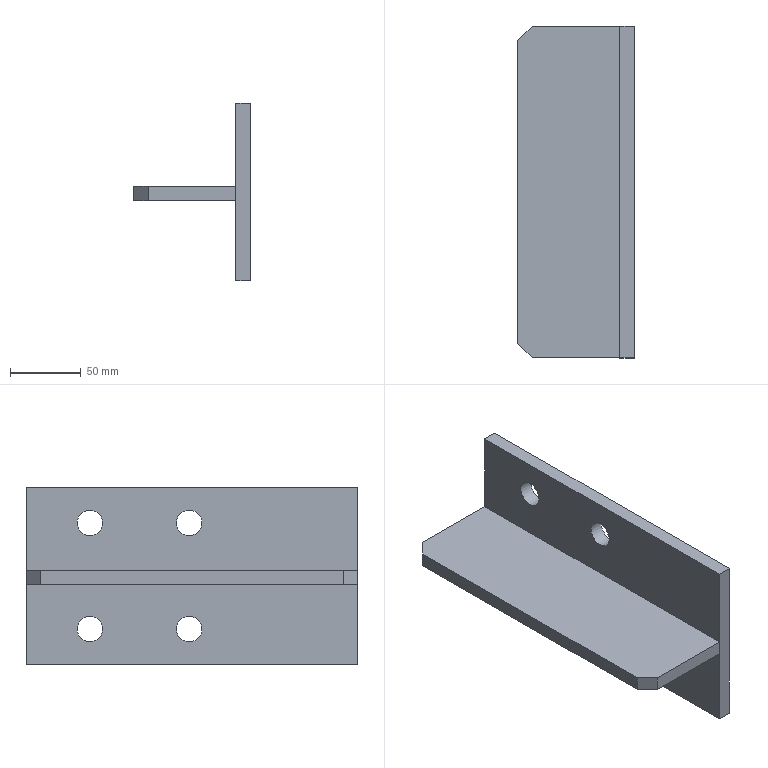Part | STEP file | PN_0030 stair beam corbel 10t_Default<As Machined> | 2 solids | 18 faces | box 82 x 234 x 125 mm | volume 449801 mm3 | plane 14 | cylinder 4 | commonest cylinder face diameters 18 x4
STEP:
#1=CARTESIAN_POINT('',(0.,0.,0.));
#2=DIRECTION('',(0.,0.,1.));
#3=DIRECTION('',(1.,0.,0.));
#4=AXIS2_PLACEMENT_3D('',#1,#2,#3);
#5=CARTESIAN_POINT('',(-26.,117.,0.));
#6=VERTEX_POINT('',#5);
#7=CARTESIAN_POINT('',(-26.,117.,10.));
#8=VERTEX_POINT('',#7);
#9=CARTESIAN_POINT('',(-26.,117.,10.));
#10=DIRECTION('',(0.,0.,1.));
#11=VECTOR('',#10,1.);
#12=LINE('',#9,#11);
#13=CARTESIAN_POINT('',(-26.,117.,10.));
#14=DIRECTION('',(0.7071,-0.7071,0.));
#15=DIRECTION('',(0.,0.,1.));
#16=AXIS2_PLACEMENT_3D('',#13,#14,#15);
#17=PLANE('',#16);
#18=CARTESIAN_POINT('',(0.,0.));
#19=DIRECTION('',(1.,0.));
#20=VECTOR('',#19,1.);
#21=LINE('',#18,#20);
#22=(GEOMETRIC_REPRESENTATION_CONTEXT(2)PARAMETRIC_REPRESENTATION_CONTEXT()REPRESENTATION_CONTEXT('',''));
#23=DEFINITIONAL_REPRESENTATION('',(#21),#22);
#24=PCURVE('',#17,#23);
#25=CARTESIAN_POINT('',(-36.,117.,10.));
#26=DIRECTION('',(0.,-1.,0.));
#27=DIRECTION('',(0.,0.,-1.));
#28=AXIS2_PLACEMENT_3D('',#25,#26,#27);
#29=PLANE('',#28);
#30=CARTESIAN_POINT('',(0.,10.));
#31=DIRECTION('',(-1.,0.));
#32=VECTOR('',#31,1.);
#33=LINE('',#30,#32);
#34=(GEOMETRIC_REPRESENTATION_CONTEXT(2)PARAMETRIC_REPRESENTATION_CONTEXT()REPRESENTATION_CONTEXT('',''));
#35=DEFINITIONAL_REPRESENTATION('',(#33),#34);
#36=PCURVE('',#29,#35);
#37=SURFACE_CURVE('',#12,(#24,#36),.PCURVE_S1.);
#38=EDGE_CURVE('',#6,#8,#37,.T.);
#39=ORIENTED_EDGE('',*,*,#38,.F.);
#40=CARTESIAN_POINT('',(-36.,107.,0.));
#41=VERTEX_POINT('',#40);
#42=CARTESIAN_POINT('',(-26.,117.,0.));
#43=DIRECTION('',(0.7071,0.7071,0.));
#44=VECTOR('',#43,1.);
#45=LINE('',#42,#44);
#46=CARTESIAN_POINT('',(-10.,0.));
#47=DIRECTION('',(0.,-1.));
#48=VECTOR('',#47,1.);
#49=LINE('',#46,#48);
#50=(GEOMETRIC_REPRESENTATION_CONTEXT(2)PARAMETRIC_REPRESENTATION_CONTEXT()REPRESENTATION_CONTEXT('',''));
#51=DEFINITIONAL_REPRESENTATION('',(#49),#50);
#52=PCURVE('',#17,#51);
#53=CARTESIAN_POINT('',(0.,0.,0.));
#54=DIRECTION('',(0.,0.,1.));
#55=DIRECTION('',(1.,0.,0.));
#56=AXIS2_PLACEMENT_3D('',#53,#54,#55);
#57=PLANE('',#56);
#58=CARTESIAN_POINT('',(-26.,117.));
#59=DIRECTION('',(0.7071,0.7071));
#60=VECTOR('',#59,1.);
#61=LINE('',#58,#60);
#62=(GEOMETRIC_REPRESENTATION_CONTEXT(2)PARAMETRIC_REPRESENTATION_CONTEXT()REPRESENTATION_CONTEXT('',''));
#63=DEFINITIONAL_REPRESENTATION('',(#61),#62);
#64=PCURVE('',#57,#63);
#65=SURFACE_CURVE('',#45,(#52,#64),.PCURVE_S1.);
#66=EDGE_CURVE('',#41,#6,#65,.T.);
#67=ORIENTED_EDGE('',*,*,#66,.F.);
#68=CARTESIAN_POINT('',(-36.,107.,10.));
#69=VERTEX_POINT('',#68);
#70=CARTESIAN_POINT('',(-36.,107.,10.));
#71=DIRECTION('',(0.,0.,-1.));
#72=VECTOR('',#71,1.);
#73=LINE('',#70,#72);
#74=CARTESIAN_POINT('',(0.,14.142));
#75=DIRECTION('',(-1.,0.));
#76=VECTOR('',#75,1.);
#77=LINE('',#74,#76);
#78=(GEOMETRIC_REPRESENTATION_CONTEXT(2)PARAMETRIC_REPRESENTATION_CONTEXT()REPRESENTATION_CONTEXT('',''));
#79=DEFINITIONAL_REPRESENTATION('',(#77),#78);
#80=PCURVE('',#17,#79);
#81=CARTESIAN_POINT('',(-36.,117.,10.));
#82=DIRECTION('',(1.,0.,0.));
#83=DIRECTION('',(0.,0.,-1.));
#84=AXIS2_PLACEMENT_3D('',#81,#82,#83);
#85=PLANE('',#84);
#86=CARTESIAN_POINT('',(0.,-10.));
#87=DIRECTION('',(1.,0.));
#88=VECTOR('',#87,1.);
#89=LINE('',#86,#88);
#90=(GEOMETRIC_REPRESENTATION_CONTEXT(2)PARAMETRIC_REPRESENTATION_CONTEXT()REPRESENTATION_CONTEXT('',''));
#91=DEFINITIONAL_REPRESENTATION('',(#89),#90);
#92=PCURVE('',#85,#91);
#93=SURFACE_CURVE('',#73,(#80,#92),.PCURVE_S1.);
#94=EDGE_CURVE('',#69,#41,#93,.T.);
#95=ORIENTED_EDGE('',*,*,#94,.F.);
#96=CARTESIAN_POINT('',(-71.5,71.5,10.));
#97=DIRECTION('',(-0.7071,-0.7071,0.));
#98=VECTOR('',#97,1.);
#99=LINE('',#96,#98);
#100=CARTESIAN_POINT('',(0.,64.347));
#101=DIRECTION('',(0.,1.));
#102=VECTOR('',#101,1.);
#103=LINE('',#100,#102);
#104=(GEOMETRIC_REPRESENTATION_CONTEXT(2)PARAMETRIC_REPRESENTATION_CONTEXT()REPRESENTATION_CONTEXT('',''));
#105=DEFINITIONAL_REPRESENTATION('',(#103),#104);
#106=PCURVE('',#17,#105);
#107=CARTESIAN_POINT('',(0.,0.,10.));
#108=DIRECTION('',(0.,0.,1.));
#109=DIRECTION('',(1.,0.,0.));
#110=AXIS2_PLACEMENT_3D('',#107,#108,#109);
#111=PLANE('',#110);
#112=CARTESIAN_POINT('',(-71.5,71.5));
#113=DIRECTION('',(-0.7071,-0.7071));
#114=VECTOR('',#113,1.);
#115=LINE('',#112,#114);
#116=(GEOMETRIC_REPRESENTATION_CONTEXT(2)PARAMETRIC_REPRESENTATION_CONTEXT()REPRESENTATION_CONTEXT('',''));
#117=DEFINITIONAL_REPRESENTATION('',(#115),#116);
#118=PCURVE('',#111,#117);
#119=SURFACE_CURVE('',#99,(#106,#118),.PCURVE_S1.);
#120=EDGE_CURVE('',#8,#69,#119,.T.);
#121=ORIENTED_EDGE('',*,*,#120,.F.);
#122=EDGE_LOOP('',(#39,#67,#95,#121));
#123=FACE_BOUND('',#122,.T.);
#124=ADVANCED_FACE('',(#123),#17,.F.);
#125=CARTESIAN_POINT('',(-36.,-107.,0.));
#126=VERTEX_POINT('',#125);
#127=CARTESIAN_POINT('',(-36.,-107.,10.));
#128=VERTEX_POINT('',#127);
#129=CARTESIAN_POINT('',(-36.,-107.,10.));
#130=DIRECTION('',(0.,0.,1.));
#131=VECTOR('',#130,1.);
#132=LINE('',#129,#131);
#133=CARTESIAN_POINT('',(-36.,-107.,10.));
#134=DIRECTION('',(0.7071,0.7071,0.));
#135=DIRECTION('',(0.,0.,1.));
#136=AXIS2_PLACEMENT_3D('',#133,#134,#135);
#137=PLANE('',#136);
#138=CARTESIAN_POINT('',(0.,0.));
#139=DIRECTION('',(1.,0.));
#140=VECTOR('',#139,1.);
#141=LINE('',#138,#140);
#142=(GEOMETRIC_REPRESENTATION_CONTEXT(2)PARAMETRIC_REPRESENTATION_CONTEXT()REPRESENTATION_CONTEXT('',''));
#143=DEFINITIONAL_REPRESENTATION('',(#141),#142);
#144=PCURVE('',#137,#143);
#145=CARTESIAN_POINT('',(0.,-224.));
#146=DIRECTION('',(-1.,0.));
#147=VECTOR('',#146,1.);
#148=LINE('',#145,#147);
#149=(GEOMETRIC_REPRESENTATION_CONTEXT(2)PARAMETRIC_REPRESENTATION_CONTEXT()REPRESENTATION_CONTEXT('',''));
#150=DEFINITIONAL_REPRESENTATION('',(#148),#149);
#151=PCURVE('',#85,#150);
#152=SURFACE_CURVE('',#132,(#144,#151),.PCURVE_S1.);
#153=EDGE_CURVE('',#126,#128,#152,.T.);
#154=ORIENTED_EDGE('',*,*,#153,.F.);
#155=CARTESIAN_POINT('',(-26.,-117.,0.));
#156=VERTEX_POINT('',#155);
#157=CARTESIAN_POINT('',(-36.,-107.,0.));
#158=DIRECTION('',(-0.7071,0.7071,0.));
#159=VECTOR('',#158,1.);
#160=LINE('',#157,#159);
#161=CARTESIAN_POINT('',(-10.,0.));
#162=DIRECTION('',(0.,-1.));
#163=VECTOR('',#162,1.);
#164=LINE('',#161,#163);
#165=(GEOMETRIC_REPRESENTATION_CONTEXT(2)PARAMETRIC_REPRESENTATION_CONTEXT()REPRESENTATION_CONTEXT('',''));
#166=DEFINITIONAL_REPRESENTATION('',(#164),#165);
#167=PCURVE('',#137,#166);
#168=CARTESIAN_POINT('',(-36.,-107.));
#169=DIRECTION('',(-0.7071,0.7071));
#170=VECTOR('',#169,1.);
#171=LINE('',#168,#170);
#172=(GEOMETRIC_REPRESENTATION_CONTEXT(2)PARAMETRIC_REPRESENTATION_CONTEXT()REPRESENTATION_CONTEXT('',''));
#173=DEFINITIONAL_REPRESENTATION('',(#171),#172);
#174=PCURVE('',#57,#173);
#175=SURFACE_CURVE('',#160,(#167,#174),.PCURVE_S1.);
#176=EDGE_CURVE('',#156,#126,#175,.T.);
#177=ORIENTED_EDGE('',*,*,#176,.F.);
#178=CARTESIAN_POINT('',(-26.,-117.,10.));
#179=VERTEX_POINT('',#178);
#180=CARTESIAN_POINT('',(-26.,-117.,10.));
#181=DIRECTION('',(0.,0.,-1.));
#182=VECTOR('',#181,1.);
#183=LINE('',#180,#182);
#184=CARTESIAN_POINT('',(0.,14.142));
#185=DIRECTION('',(-1.,0.));
#186=VECTOR('',#185,1.);
#187=LINE('',#184,#186);
#188=(GEOMETRIC_REPRESENTATION_CONTEXT(2)PARAMETRIC_REPRESENTATION_CONTEXT()REPRESENTATION_CONTEXT('',''));
#189=DEFINITIONAL_REPRESENTATION('',(#187),#188);
#190=PCURVE('',#137,#189);
#191=CARTESIAN_POINT('',(-36.,-117.,10.));
#192=DIRECTION('',(0.,1.,0.));
#193=DIRECTION('',(0.,0.,1.));
#194=AXIS2_PLACEMENT_3D('',#191,#192,#193);
#195=PLANE('',#194);
#196=CARTESIAN_POINT('',(0.,10.));
#197=DIRECTION('',(-1.,0.));
#198=VECTOR('',#197,1.);
#199=LINE('',#196,#198);
#200=(GEOMETRIC_REPRESENTATION_CONTEXT(2)PARAMETRIC_REPRESENTATION_CONTEXT()REPRESENTATION_CONTEXT('',''));
#201=DEFINITIONAL_REPRESENTATION('',(#199),#200);
#202=PCURVE('',#195,#201);
#203=SURFACE_CURVE('',#183,(#190,#202),.PCURVE_S1.);
#204=EDGE_CURVE('',#179,#156,#203,.T.);
#205=ORIENTED_EDGE('',*,*,#204,.F.);
#206=CARTESIAN_POINT('',(-71.5,-71.5,10.));
#207=DIRECTION('',(0.7071,-0.7071,0.));
#208=VECTOR('',#207,1.);
#209=LINE('',#206,#208);
#210=CARTESIAN_POINT('',(0.,-50.205));
#211=DIRECTION('',(0.,1.));
#212=VECTOR('',#211,1.);
#213=LINE('',#210,#212);
#214=(GEOMETRIC_REPRESENTATION_CONTEXT(2)PARAMETRIC_REPRESENTATION_CONTEXT()REPRESENTATION_CONTEXT('',''));
#215=DEFINITIONAL_REPRESENTATION('',(#213),#214);
#216=PCURVE('',#137,#215);
#217=CARTESIAN_POINT('',(-71.5,-71.5));
#218=DIRECTION('',(0.7071,-0.7071));
#219=VECTOR('',#218,1.);
#220=LINE('',#217,#219);
#221=(GEOMETRIC_REPRESENTATION_CONTEXT(2)PARAMETRIC_REPRESENTATION_CONTEXT()REPRESENTATION_CONTEXT('',''));
#222=DEFINITIONAL_REPRESENTATION('',(#220),#221);
#223=PCURVE('',#111,#222);
#224=SURFACE_CURVE('',#209,(#216,#223),.PCURVE_S1.);
#225=EDGE_CURVE('',#128,#179,#224,.T.);
#226=ORIENTED_EDGE('',*,*,#225,.F.);
#227=EDGE_LOOP('',(#154,#177,#205,#226));
#228=FACE_BOUND('',#227,.T.);
#229=ADVANCED_FACE('',(#228),#137,.F.);
#230=CARTESIAN_POINT('',(36.,-117.,0.));
#231=VERTEX_POINT('',#230);
#232=CARTESIAN_POINT('',(36.,117.,0.));
#233=VERTEX_POINT('',#232);
#234=CARTESIAN_POINT('',(36.,117.,0.));
#235=DIRECTION('',(0.,1.,0.));
#236=VECTOR('',#235,1.);
#237=LINE('',#234,#236);
#238=CARTESIAN_POINT('',(36.,117.,10.));
#239=DIRECTION('',(-1.,0.,0.));
#240=DIRECTION('',(0.,0.,1.));
#241=AXIS2_PLACEMENT_3D('',#238,#239,#240);
#242=PLANE('',#241);
#243=CARTESIAN_POINT('',(-10.,0.));
#244=DIRECTION('',(0.,1.));
#245=VECTOR('',#244,1.);
#246=LINE('',#243,#245);
#247=(GEOMETRIC_REPRESENTATION_CONTEXT(2)PARAMETRIC_REPRESENTATION_CONTEXT()REPRESENTATION_CONTEXT('',''));
#248=DEFINITIONAL_REPRESENTATION('',(#246),#247);
#249=PCURVE('',#242,#248);
#250=CARTESIAN_POINT('',(36.,117.));
#251=DIRECTION('',(0.,1.));
#252=VECTOR('',#251,1.);
#253=LINE('',#250,#252);
#254=(GEOMETRIC_REPRESENTATION_CONTEXT(2)PARAMETRIC_REPRESENTATION_CONTEXT()REPRESENTATION_CONTEXT('',''));
#255=DEFINITIONAL_REPRESENTATION('',(#253),#254);
#256=PCURVE('',#57,#255);
#257=SURFACE_CURVE('',#237,(#249,#256),.PCURVE_S1.);
#258=EDGE_CURVE('',#231,#233,#257,.T.);
#259=ORIENTED_EDGE('',*,*,#258,.T.);
#260=CARTESIAN_POINT('',(36.,117.,10.));
#261=VERTEX_POINT('',#260);
#262=CARTESIAN_POINT('',(36.,117.,10.));
#263=DIRECTION('',(0.,0.,-1.));
#264=VECTOR('',#263,1.);
#265=LINE('',#262,#264);
#266=CARTESIAN_POINT('',(0.,0.));
#267=DIRECTION('',(-1.,0.));
#268=VECTOR('',#267,1.);
#269=LINE('',#266,#268);
#270=(GEOMETRIC_REPRESENTATION_CONTEXT(2)PARAMETRIC_REPRESENTATION_CONTEXT()REPRESENTATION_CONTEXT('',''));
#271=DEFINITIONAL_REPRESENTATION('',(#269),#270);
#272=PCURVE('',#242,#271);
#273=CARTESIAN_POINT('',(0.,72.));
#274=DIRECTION('',(1.,0.));
#275=VECTOR('',#274,1.);
#276=LINE('',#273,#275);
#277=(GEOMETRIC_REPRESENTATION_CONTEXT(2)PARAMETRIC_REPRESENTATION_CONTEXT()REPRESENTATION_CONTEXT('',''));
#278=DEFINITIONAL_REPRESENTATION('',(#276),#277);
#279=PCURVE('',#29,#278);
#280=SURFACE_CURVE('',#265,(#272,#279),.PCURVE_S1.);
#281=EDGE_CURVE('',#261,#233,#280,.T.);
#282=ORIENTED_EDGE('',*,*,#281,.F.);
#283=CARTESIAN_POINT('',(36.,-117.,10.));
#284=VERTEX_POINT('',#283);
#285=CARTESIAN_POINT('',(36.,117.,10.));
#286=DIRECTION('',(0.,1.,0.));
#287=VECTOR('',#286,1.);
#288=LINE('',#285,#287);
#289=CARTESIAN_POINT('',(0.,0.));
#290=DIRECTION('',(0.,1.));
#291=VECTOR('',#290,1.);
#292=LINE('',#289,#291);
#293=(GEOMETRIC_REPRESENTATION_CONTEXT(2)PARAMETRIC_REPRESENTATION_CONTEXT()REPRESENTATION_CONTEXT('',''));
#294=DEFINITIONAL_REPRESENTATION('',(#292),#293);
#295=PCURVE('',#242,#294);
#296=CARTESIAN_POINT('',(36.,117.));
#297=DIRECTION('',(0.,1.));
#298=VECTOR('',#297,1.);
#299=LINE('',#296,#298);
#300=(GEOMETRIC_REPRESENTATION_CONTEXT(2)PARAMETRIC_REPRESENTATION_CONTEXT()REPRESENTATION_CONTEXT('',''));
#301=DEFINITIONAL_REPRESENTATION('',(#299),#300);
#302=PCURVE('',#111,#301);
#303=SURFACE_CURVE('',#288,(#295,#302),.PCURVE_S1.);
#304=EDGE_CURVE('',#284,#261,#303,.T.);
#305=ORIENTED_EDGE('',*,*,#304,.F.);
#306=CARTESIAN_POINT('',(36.,-117.,10.));
#307=DIRECTION('',(0.,0.,-1.));
#308=VECTOR('',#307,1.);
#309=LINE('',#306,#308);
#310=CARTESIAN_POINT('',(0.,-234.));
#311=DIRECTION('',(-1.,0.));
#312=VECTOR('',#311,1.);
#313=LINE('',#310,#312);
#314=(GEOMETRIC_REPRESENTATION_CONTEXT(2)PARAMETRIC_REPRESENTATION_CONTEXT()REPRESENTATION_CONTEXT('',''));
#315=DEFINITIONAL_REPRESENTATION('',(#313),#314);
#316=PCURVE('',#242,#315);
#317=CARTESIAN_POINT('',(0.,72.));
#318=DIRECTION('',(-1.,0.));
#319=VECTOR('',#318,1.);
#320=LINE('',#317,#319);
#321=(GEOMETRIC_REPRESENTATION_CONTEXT(2)PARAMETRIC_REPRESENTATION_CONTEXT()REPRESENTATION_CONTEXT('',''));
#322=DEFINITIONAL_REPRESENTATION('',(#320),#321);
#323=PCURVE('',#195,#322);
#324=SURFACE_CURVE('',#309,(#316,#323),.PCURVE_S1.);
#325=EDGE_CURVE('',#284,#231,#324,.T.);
#326=ORIENTED_EDGE('',*,*,#325,.T.);
#327=EDGE_LOOP('',(#259,#282,#305,#326));
#328=FACE_BOUND('',#327,.T.);
#329=ADVANCED_FACE('',(#328),#242,.F.);
#330=CARTESIAN_POINT('',(-36.,117.,0.));
#331=DIRECTION('',(-1.,0.,0.));
#332=VECTOR('',#331,1.);
#333=LINE('',#330,#332);
#334=CARTESIAN_POINT('',(10.,0.));
#335=DIRECTION('',(0.,-1.));
#336=VECTOR('',#335,1.);
#337=LINE('',#334,#336);
#338=(GEOMETRIC_REPRESENTATION_CONTEXT(2)PARAMETRIC_REPRESENTATION_CONTEXT()REPRESENTATION_CONTEXT('',''));
#339=DEFINITIONAL_REPRESENTATION('',(#337),#338);
#340=PCURVE('',#29,#339);
#341=CARTESIAN_POINT('',(-36.,117.));
#342=DIRECTION('',(-1.,0.));
#343=VECTOR('',#342,1.);
#344=LINE('',#341,#343);
#345=(GEOMETRIC_REPRESENTATION_CONTEXT(2)PARAMETRIC_REPRESENTATION_CONTEXT()REPRESENTATION_CONTEXT('',''));
#346=DEFINITIONAL_REPRESENTATION('',(#344),#345);
#347=PCURVE('',#57,#346);
#348=SURFACE_CURVE('',#333,(#340,#347),.PCURVE_S1.);
#349=EDGE_CURVE('',#233,#6,#348,.T.);
#350=ORIENTED_EDGE('',*,*,#349,.T.);
#351=ORIENTED_EDGE('',*,*,#38,.T.);
#352=CARTESIAN_POINT('',(-36.,117.,10.));
#353=DIRECTION('',(-1.,0.,0.));
#354=VECTOR('',#353,1.);
#355=LINE('',#352,#354);
#356=CARTESIAN_POINT('',(0.,0.));
#357=DIRECTION('',(0.,-1.));
#358=VECTOR('',#357,1.);
#359=LINE('',#356,#358);
#360=(GEOMETRIC_REPRESENTATION_CONTEXT(2)PARAMETRIC_REPRESENTATION_CONTEXT()REPRESENTATION_CONTEXT('',''));
#361=DEFINITIONAL_REPRESENTATION('',(#359),#360);
#362=PCURVE('',#29,#361);
#363=CARTESIAN_POINT('',(-36.,117.));
#364=DIRECTION('',(-1.,0.));
#365=VECTOR('',#364,1.);
#366=LINE('',#363,#365);
#367=(GEOMETRIC_REPRESENTATION_CONTEXT(2)PARAMETRIC_REPRESENTATION_CONTEXT()REPRESENTATION_CONTEXT('',''));
#368=DEFINITIONAL_REPRESENTATION('',(#366),#367);
#369=PCURVE('',#111,#368);
#370=SURFACE_CURVE('',#355,(#362,#369),.PCURVE_S1.);
#371=EDGE_CURVE('',#261,#8,#370,.T.);
#372=ORIENTED_EDGE('',*,*,#371,.F.);
#373=ORIENTED_EDGE('',*,*,#281,.T.);
#374=EDGE_LOOP('',(#350,#351,#372,#373));
#375=FACE_BOUND('',#374,.T.);
#376=ADVANCED_FACE('',(#375),#29,.F.);
#377=CARTESIAN_POINT('',(-36.,117.,10.));
#378=DIRECTION('',(0.,-1.,0.));
#379=VECTOR('',#378,1.);
#380=LINE('',#377,#379);
#381=CARTESIAN_POINT('',(0.,0.));
#382=DIRECTION('',(0.,-1.));
#383=VECTOR('',#382,1.);
#384=LINE('',#381,#383);
#385=(GEOMETRIC_REPRESENTATION_CONTEXT(2)PARAMETRIC_REPRESENTATION_CONTEXT()REPRESENTATION_CONTEXT('',''));
#386=DEFINITIONAL_REPRESENTATION('',(#384),#385);
#387=PCURVE('',#85,#386);
#388=CARTESIAN_POINT('',(-36.,117.));
#389=DIRECTION('',(0.,-1.));
#390=VECTOR('',#389,1.);
#391=LINE('',#388,#390);
#392=(GEOMETRIC_REPRESENTATION_CONTEXT(2)PARAMETRIC_REPRESENTATION_CONTEXT()REPRESENTATION_CONTEXT('',''));
#393=DEFINITIONAL_REPRESENTATION('',(#391),#392);
#394=PCURVE('',#111,#393);
#395=SURFACE_CURVE('',#380,(#387,#394),.PCURVE_S1.);
#396=EDGE_CURVE('',#69,#128,#395,.T.);
#397=ORIENTED_EDGE('',*,*,#396,.F.);
#398=ORIENTED_EDGE('',*,*,#94,.T.);
#399=CARTESIAN_POINT('',(-36.,117.,0.));
#400=DIRECTION('',(0.,-1.,0.));
#401=VECTOR('',#400,1.);
#402=LINE('',#399,#401);
#403=CARTESIAN_POINT('',(10.,0.));
#404=DIRECTION('',(0.,-1.));
#405=VECTOR('',#404,1.);
#406=LINE('',#403,#405);
#407=(GEOMETRIC_REPRESENTATION_CONTEXT(2)PARAMETRIC_REPRESENTATION_CONTEXT()REPRESENTATION_CONTEXT('',''));
#408=DEFINITIONAL_REPRESENTATION('',(#406),#407);
#409=PCURVE('',#85,#408);
#410=CARTESIAN_POINT('',(-36.,117.));
#411=DIRECTION('',(0.,-1.));
#412=VECTOR('',#411,1.);
#413=LINE('',#410,#412);
#414=(GEOMETRIC_REPRESENTATION_CONTEXT(2)PARAMETRIC_REPRESENTATION_CONTEXT()REPRESENTATION_CONTEXT('',''));
#415=DEFINITIONAL_REPRESENTATION('',(#413),#414);
#416=PCURVE('',#57,#415);
#417=SURFACE_CURVE('',#402,(#409,#416),.PCURVE_S1.);
#418=EDGE_CURVE('',#41,#126,#417,.T.);
#419=ORIENTED_EDGE('',*,*,#418,.T.);
#420=ORIENTED_EDGE('',*,*,#153,.T.);
#421=EDGE_LOOP('',(#397,#398,#419,#420));
#422=FACE_BOUND('',#421,.T.);
#423=ADVANCED_FACE('',(#422),#85,.F.);
#424=CARTESIAN_POINT('',(-36.,-117.,10.));
#425=DIRECTION('',(1.,0.,0.));
#426=VECTOR('',#425,1.);
#427=LINE('',#424,#426);
#428=CARTESIAN_POINT('',(0.,0.));
#429=DIRECTION('',(0.,1.));
#430=VECTOR('',#429,1.);
#431=LINE('',#428,#430);
#432=(GEOMETRIC_REPRESENTATION_CONTEXT(2)PARAMETRIC_REPRESENTATION_CONTEXT()REPRESENTATION_CONTEXT('',''));
#433=DEFINITIONAL_REPRESENTATION('',(#431),#432);
#434=PCURVE('',#195,#433);
#435=CARTESIAN_POINT('',(-36.,-117.));
#436=DIRECTION('',(1.,0.));
#437=VECTOR('',#436,1.);
#438=LINE('',#435,#437);
#439=(GEOMETRIC_REPRESENTATION_CONTEXT(2)PARAMETRIC_REPRESENTATION_CONTEXT()REPRESENTATION_CONTEXT('',''));
#440=DEFINITIONAL_REPRESENTATION('',(#438),#439);
#441=PCURVE('',#111,#440);
#442=SURFACE_CURVE('',#427,(#434,#441),.PCURVE_S1.);
#443=EDGE_CURVE('',#179,#284,#442,.T.);
#444=ORIENTED_EDGE('',*,*,#443,.F.);
#445=ORIENTED_EDGE('',*,*,#204,.T.);
#446=CARTESIAN_POINT('',(-36.,-117.,0.));
#447=DIRECTION('',(1.,0.,0.));
#448=VECTOR('',#447,1.);
#449=LINE('',#446,#448);
#450=CARTESIAN_POINT('',(-10.,0.));
#451=DIRECTION('',(0.,1.));
#452=VECTOR('',#451,1.);
#453=LINE('',#450,#452);
#454=(GEOMETRIC_REPRESENTATION_CONTEXT(2)PARAMETRIC_REPRESENTATION_CONTEXT()REPRESENTATION_CONTEXT('',''));
#455=DEFINITIONAL_REPRESENTATION('',(#453),#454);
#456=PCURVE('',#195,#455);
#457=CARTESIAN_POINT('',(-36.,-117.));
#458=DIRECTION('',(1.,0.));
#459=VECTOR('',#458,1.);
#460=LINE('',#457,#459);
#461=(GEOMETRIC_REPRESENTATION_CONTEXT(2)PARAMETRIC_REPRESENTATION_CONTEXT()REPRESENTATION_CONTEXT('',''));
#462=DEFINITIONAL_REPRESENTATION('',(#460),#461);
#463=PCURVE('',#57,#462);
#464=SURFACE_CURVE('',#449,(#456,#463),.PCURVE_S1.);
#465=EDGE_CURVE('',#156,#231,#464,.T.);
#466=ORIENTED_EDGE('',*,*,#465,.T.);
#467=ORIENTED_EDGE('',*,*,#325,.F.);
#468=EDGE_LOOP('',(#444,#445,#466,#467));
#469=FACE_BOUND('',#468,.T.);
#470=ADVANCED_FACE('',(#469),#195,.F.);
#471=ORIENTED_EDGE('',*,*,#371,.T.);
#472=ORIENTED_EDGE('',*,*,#120,.T.);
#473=ORIENTED_EDGE('',*,*,#396,.T.);
#474=ORIENTED_EDGE('',*,*,#225,.T.);
#475=ORIENTED_EDGE('',*,*,#443,.T.);
#476=ORIENTED_EDGE('',*,*,#304,.T.);
#477=EDGE_LOOP('',(#471,#472,#473,#474,#475,#476));
#478=FACE_BOUND('',#477,.T.);
#479=ADVANCED_FACE('',(#478),#111,.T.);
#480=ORIENTED_EDGE('',*,*,#418,.F.);
#481=ORIENTED_EDGE('',*,*,#66,.T.);
#482=ORIENTED_EDGE('',*,*,#349,.F.);
#483=ORIENTED_EDGE('',*,*,#258,.F.);
#484=ORIENTED_EDGE('',*,*,#465,.F.);
#485=ORIENTED_EDGE('',*,*,#176,.T.);
#486=EDGE_LOOP('',(#480,#481,#482,#483,#484,#485));
#487=FACE_BOUND('',#486,.T.);
#488=ADVANCED_FACE('',(#487),#57,.F.);
#489=CLOSED_SHELL('',(#124,#229,#329,#376,#423,#470,#479,#488));
#490=MANIFOLD_SOLID_BREP('',#489);
#491=CARTESIAN_POINT('',(36.,-117.,-56.496));
#492=VERTEX_POINT('',#491);
#493=CARTESIAN_POINT('',(36.,117.,-56.496));
#494=VERTEX_POINT('',#493);
#495=CARTESIAN_POINT('',(36.,117.,-56.496));
#496=DIRECTION('',(0.,1.,0.));
#497=VECTOR('',#496,1.);
#498=LINE('',#495,#497);
#499=CARTESIAN_POINT('',(46.,117.,-56.496));
#500=DIRECTION('',(0.,0.,1.));
#501=DIRECTION('',(1.,0.,0.));
#502=AXIS2_PLACEMENT_3D('',#499,#500,#501);
#503=PLANE('',#502);
#504=CARTESIAN_POINT('',(-10.,0.));
#505=DIRECTION('',(0.,1.));
#506=VECTOR('',#505,1.);
#507=LINE('',#504,#506);
#508=(GEOMETRIC_REPRESENTATION_CONTEXT(2)PARAMETRIC_REPRESENTATION_CONTEXT()REPRESENTATION_CONTEXT('',''));
#509=DEFINITIONAL_REPRESENTATION('',(#507),#508);
#510=PCURVE('',#503,#509);
#511=CARTESIAN_POINT('',(36.,-17.06,106.06));
#512=DIRECTION('',(1.,0.,0.));
#513=DIRECTION('',(0.,0.,-1.));
#514=AXIS2_PLACEMENT_3D('',#511,#512,#513);
#515=PLANE('',#514);
#516=CARTESIAN_POINT('',(162.556,134.06));
#517=DIRECTION('',(0.,1.));
#518=VECTOR('',#517,1.);
#519=LINE('',#516,#518);
#520=(GEOMETRIC_REPRESENTATION_CONTEXT(2)PARAMETRIC_REPRESENTATION_CONTEXT()REPRESENTATION_CONTEXT('',''));
#521=DEFINITIONAL_REPRESENTATION('',(#519),#520);
#522=PCURVE('',#515,#521);
#523=SURFACE_CURVE('',#498,(#510,#522),.PCURVE_S1.);
#524=EDGE_CURVE('',#492,#494,#523,.T.);
#525=ORIENTED_EDGE('',*,*,#524,.T.);
#526=CARTESIAN_POINT('',(46.,117.,-56.496));
#527=VERTEX_POINT('',#526);
#528=CARTESIAN_POINT('',(46.,117.,-56.496));
#529=DIRECTION('',(-1.,0.,0.));
#530=VECTOR('',#529,1.);
#531=LINE('',#528,#530);
#532=CARTESIAN_POINT('',(0.,0.));
#533=DIRECTION('',(-1.,0.));
#534=VECTOR('',#533,1.);
#535=LINE('',#532,#534);
#536=(GEOMETRIC_REPRESENTATION_CONTEXT(2)PARAMETRIC_REPRESENTATION_CONTEXT()REPRESENTATION_CONTEXT('',''));
#537=DEFINITIONAL_REPRESENTATION('',(#535),#536);
#538=PCURVE('',#503,#537);
#539=CARTESIAN_POINT('',(46.,117.,68.504));
#540=DIRECTION('',(0.,-1.,0.));
#541=DIRECTION('',(0.,0.,-1.));
#542=AXIS2_PLACEMENT_3D('',#539,#540,#541);
#543=PLANE('',#542);
#544=CARTESIAN_POINT('',(125.,0.));
#545=DIRECTION('',(0.,-1.));
#546=VECTOR('',#545,1.);
#547=LINE('',#544,#546);
#548=(GEOMETRIC_REPRESENTATION_CONTEXT(2)PARAMETRIC_REPRESENTATION_CONTEXT()REPRESENTATION_CONTEXT('',''));
#549=DEFINITIONAL_REPRESENTATION('',(#547),#548);
#550=PCURVE('',#543,#549);
#551=SURFACE_CURVE('',#531,(#538,#550),.PCURVE_S1.);
#552=EDGE_CURVE('',#527,#494,#551,.T.);
#553=ORIENTED_EDGE('',*,*,#552,.F.);
#554=CARTESIAN_POINT('',(46.,-117.,-56.496));
#555=VERTEX_POINT('',#554);
#556=CARTESIAN_POINT('',(46.,117.,-56.496));
#557=DIRECTION('',(0.,1.,0.));
#558=VECTOR('',#557,1.);
#559=LINE('',#556,#558);
#560=CARTESIAN_POINT('',(0.,0.));
#561=DIRECTION('',(0.,1.));
#562=VECTOR('',#561,1.);
#563=LINE('',#560,#562);
#564=(GEOMETRIC_REPRESENTATION_CONTEXT(2)PARAMETRIC_REPRESENTATION_CONTEXT()REPRESENTATION_CONTEXT('',''));
#565=DEFINITIONAL_REPRESENTATION('',(#563),#564);
#566=PCURVE('',#503,#565);
#567=CARTESIAN_POINT('',(46.,-17.06,106.06));
#568=DIRECTION('',(1.,0.,0.));
#569=DIRECTION('',(0.,0.,-1.));
#570=AXIS2_PLACEMENT_3D('',#567,#568,#569);
#571=PLANE('',#570);
#572=CARTESIAN_POINT('',(162.556,134.06));
#573=DIRECTION('',(0.,1.));
#574=VECTOR('',#573,1.);
#575=LINE('',#572,#574);
#576=(GEOMETRIC_REPRESENTATION_CONTEXT(2)PARAMETRIC_REPRESENTATION_CONTEXT()REPRESENTATION_CONTEXT('',''));
#577=DEFINITIONAL_REPRESENTATION('',(#575),#576);
#578=PCURVE('',#571,#577);
#579=SURFACE_CURVE('',#559,(#566,#578),.PCURVE_S1.);
#580=EDGE_CURVE('',#555,#527,#579,.T.);
#581=ORIENTED_EDGE('',*,*,#580,.F.);
#582=CARTESIAN_POINT('',(46.,-117.,-56.496));
#583=DIRECTION('',(-1.,0.,0.));
#584=VECTOR('',#583,1.);
#585=LINE('',#582,#584);
#586=CARTESIAN_POINT('',(0.,-234.));
#587=DIRECTION('',(-1.,0.));
#588=VECTOR('',#587,1.);
#589=LINE('',#586,#588);
#590=(GEOMETRIC_REPRESENTATION_CONTEXT(2)PARAMETRIC_REPRESENTATION_CONTEXT()REPRESENTATION_CONTEXT('',''));
#591=DEFINITIONAL_REPRESENTATION('',(#589),#590);
#592=PCURVE('',#503,#591);
#593=CARTESIAN_POINT('',(46.,-117.,68.504));
#594=DIRECTION('',(0.,1.,0.));
#595=DIRECTION('',(0.,0.,1.));
#596=AXIS2_PLACEMENT_3D('',#593,#594,#595);
#597=PLANE('',#596);
#598=CARTESIAN_POINT('',(-125.,0.));
#599=DIRECTION('',(0.,-1.));
#600=VECTOR('',#599,1.);
#601=LINE('',#598,#600);
#602=(GEOMETRIC_REPRESENTATION_CONTEXT(2)PARAMETRIC_REPRESENTATION_CONTEXT()REPRESENTATION_CONTEXT('',''));
#603=DEFINITIONAL_REPRESENTATION('',(#601),#602);
#604=PCURVE('',#597,#603);
#605=SURFACE_CURVE('',#585,(#592,#604),.PCURVE_S1.);
#606=EDGE_CURVE('',#555,#492,#605,.T.);
#607=ORIENTED_EDGE('',*,*,#606,.T.);
#608=EDGE_LOOP('',(#525,#553,#581,#607));
#609=FACE_BOUND('',#608,.T.);
#610=ADVANCED_FACE('',(#609),#503,.F.);
#611=CARTESIAN_POINT('',(36.,117.,68.504));
#612=VERTEX_POINT('',#611);
#613=CARTESIAN_POINT('',(36.,117.,68.504));
#614=DIRECTION('',(0.,0.,1.));
#615=VECTOR('',#614,1.);
#616=LINE('',#613,#615);
#617=CARTESIAN_POINT('',(0.,-10.));
#618=DIRECTION('',(-1.,0.));
#619=VECTOR('',#618,1.);
#620=LINE('',#617,#619);
#621=(GEOMETRIC_REPRESENTATION_CONTEXT(2)PARAMETRIC_REPRESENTATION_CONTEXT()REPRESENTATION_CONTEXT('',''));
#622=DEFINITIONAL_REPRESENTATION('',(#620),#621);
#623=PCURVE('',#543,#622);
#624=CARTESIAN_POINT('',(37.556,134.06));
#625=DIRECTION('',(-1.,0.));
#626=VECTOR('',#625,1.);
#627=LINE('',#624,#626);
#628=(GEOMETRIC_REPRESENTATION_CONTEXT(2)PARAMETRIC_REPRESENTATION_CONTEXT()REPRESENTATION_CONTEXT('',''));
#629=DEFINITIONAL_REPRESENTATION('',(#627),#628);
#630=PCURVE('',#515,#629);
#631=SURFACE_CURVE('',#616,(#623,#630),.PCURVE_S1.);
#632=EDGE_CURVE('',#494,#612,#631,.T.);
#633=ORIENTED_EDGE('',*,*,#632,.T.);
#634=CARTESIAN_POINT('',(46.,117.,68.504));
#635=VERTEX_POINT('',#634);
#636=CARTESIAN_POINT('',(46.,117.,68.504));
#637=DIRECTION('',(-1.,0.,0.));
#638=VECTOR('',#637,1.);
#639=LINE('',#636,#638);
#640=CARTESIAN_POINT('',(0.,0.));
#641=DIRECTION('',(0.,-1.));
#642=VECTOR('',#641,1.);
#643=LINE('',#640,#642);
#644=(GEOMETRIC_REPRESENTATION_CONTEXT(2)PARAMETRIC_REPRESENTATION_CONTEXT()REPRESENTATION_CONTEXT('',''));
#645=DEFINITIONAL_REPRESENTATION('',(#643),#644);
#646=PCURVE('',#543,#645);
#647=CARTESIAN_POINT('',(46.,117.,68.504));
#648=DIRECTION('',(0.,0.,-1.));
#649=DIRECTION('',(0.,1.,0.));
#650=AXIS2_PLACEMENT_3D('',#647,#648,#649);
#651=PLANE('',#650);
#652=CARTESIAN_POINT('',(0.,0.));
#653=DIRECTION('',(0.,-1.));
#654=VECTOR('',#653,1.);
#655=LINE('',#652,#654);
#656=(GEOMETRIC_REPRESENTATION_CONTEXT(2)PARAMETRIC_REPRESENTATION_CONTEXT()REPRESENTATION_CONTEXT('',''));
#657=DEFINITIONAL_REPRESENTATION('',(#655),#656);
#658=PCURVE('',#651,#657);
#659=SURFACE_CURVE('',#639,(#646,#658),.PCURVE_S1.);
#660=EDGE_CURVE('',#635,#612,#659,.T.);
#661=ORIENTED_EDGE('',*,*,#660,.F.);
#662=CARTESIAN_POINT('',(46.,117.,68.504));
#663=DIRECTION('',(0.,0.,1.));
#664=VECTOR('',#663,1.);
#665=LINE('',#662,#664);
#666=CARTESIAN_POINT('',(0.,0.));
#667=DIRECTION('',(-1.,0.));
#668=VECTOR('',#667,1.);
#669=LINE('',#666,#668);
#670=(GEOMETRIC_REPRESENTATION_CONTEXT(2)PARAMETRIC_REPRESENTATION_CONTEXT()REPRESENTATION_CONTEXT('',''));
#671=DEFINITIONAL_REPRESENTATION('',(#669),#670);
#672=PCURVE('',#543,#671);
#673=CARTESIAN_POINT('',(37.556,134.06));
#674=DIRECTION('',(-1.,0.));
#675=VECTOR('',#674,1.);
#676=LINE('',#673,#675);
#677=(GEOMETRIC_REPRESENTATION_CONTEXT(2)PARAMETRIC_REPRESENTATION_CONTEXT()REPRESENTATION_CONTEXT('',''));
#678=DEFINITIONAL_REPRESENTATION('',(#676),#677);
#679=PCURVE('',#571,#678);
#680=SURFACE_CURVE('',#665,(#672,#679),.PCURVE_S1.);
#681=EDGE_CURVE('',#527,#635,#680,.T.);
#682=ORIENTED_EDGE('',*,*,#681,.F.);
#683=ORIENTED_EDGE('',*,*,#552,.T.);
#684=EDGE_LOOP('',(#633,#661,#682,#683));
#685=FACE_BOUND('',#684,.T.);
#686=ADVANCED_FACE('',(#685),#543,.F.);
#687=CARTESIAN_POINT('',(36.,-117.,68.504));
#688=VERTEX_POINT('',#687);
#689=CARTESIAN_POINT('',(36.,117.,68.504));
#690=DIRECTION('',(0.,-1.,0.));
#691=VECTOR('',#690,1.);
#692=LINE('',#689,#691);
#693=CARTESIAN_POINT('',(0.,-10.));
#694=DIRECTION('',(-1.,0.));
#695=VECTOR('',#694,1.);
#696=LINE('',#693,#695);
#697=(GEOMETRIC_REPRESENTATION_CONTEXT(2)PARAMETRIC_REPRESENTATION_CONTEXT()REPRESENTATION_CONTEXT('',''));
#698=DEFINITIONAL_REPRESENTATION('',(#696),#697);
#699=PCURVE('',#651,#698);
#700=CARTESIAN_POINT('',(37.556,134.06));
#701=DIRECTION('',(0.,-1.));
#702=VECTOR('',#701,1.);
#703=LINE('',#700,#702);
#704=(GEOMETRIC_REPRESENTATION_CONTEXT(2)PARAMETRIC_REPRESENTATION_CONTEXT()REPRESENTATION_CONTEXT('',''));
#705=DEFINITIONAL_REPRESENTATION('',(#703),#704);
#706=PCURVE('',#515,#705);
#707=SURFACE_CURVE('',#692,(#699,#706),.PCURVE_S1.);
#708=EDGE_CURVE('',#612,#688,#707,.T.);
#709=ORIENTED_EDGE('',*,*,#708,.T.);
#710=CARTESIAN_POINT('',(46.,-117.,68.504));
#711=VERTEX_POINT('',#710);
#712=CARTESIAN_POINT('',(46.,-117.,68.504));
#713=DIRECTION('',(-1.,0.,0.));
#714=VECTOR('',#713,1.);
#715=LINE('',#712,#714);
#716=CARTESIAN_POINT('',(-234.,0.));
#717=DIRECTION('',(0.,-1.));
#718=VECTOR('',#717,1.);
#719=LINE('',#716,#718);
#720=(GEOMETRIC_REPRESENTATION_CONTEXT(2)PARAMETRIC_REPRESENTATION_CONTEXT()REPRESENTATION_CONTEXT('',''));
#721=DEFINITIONAL_REPRESENTATION('',(#719),#720);
#722=PCURVE('',#651,#721);
#723=CARTESIAN_POINT('',(0.,0.));
#724=DIRECTION('',(0.,-1.));
#725=VECTOR('',#724,1.);
#726=LINE('',#723,#725);
#727=(GEOMETRIC_REPRESENTATION_CONTEXT(2)PARAMETRIC_REPRESENTATION_CONTEXT()REPRESENTATION_CONTEXT('',''));
#728=DEFINITIONAL_REPRESENTATION('',(#726),#727);
#729=PCURVE('',#597,#728);
#730=SURFACE_CURVE('',#715,(#722,#729),.PCURVE_S1.);
#731=EDGE_CURVE('',#711,#688,#730,.T.);
#732=ORIENTED_EDGE('',*,*,#731,.F.);
#733=CARTESIAN_POINT('',(46.,117.,68.504));
#734=DIRECTION('',(0.,-1.,0.));
#735=VECTOR('',#734,1.);
#736=LINE('',#733,#735);
#737=CARTESIAN_POINT('',(0.,0.));
#738=DIRECTION('',(-1.,0.));
#739=VECTOR('',#738,1.);
#740=LINE('',#737,#739);
#741=(GEOMETRIC_REPRESENTATION_CONTEXT(2)PARAMETRIC_REPRESENTATION_CONTEXT()REPRESENTATION_CONTEXT('',''));
#742=DEFINITIONAL_REPRESENTATION('',(#740),#741);
#743=PCURVE('',#651,#742);
#744=CARTESIAN_POINT('',(37.556,134.06));
#745=DIRECTION('',(0.,-1.));
#746=VECTOR('',#745,1.);
#747=LINE('',#744,#746);
#748=(GEOMETRIC_REPRESENTATION_CONTEXT(2)PARAMETRIC_REPRESENTATION_CONTEXT()REPRESENTATION_CONTEXT('',''));
#749=DEFINITIONAL_REPRESENTATION('',(#747),#748);
#750=PCURVE('',#571,#749);
#751=SURFACE_CURVE('',#736,(#743,#750),.PCURVE_S1.);
#752=EDGE_CURVE('',#635,#711,#751,.T.);
#753=ORIENTED_EDGE('',*,*,#752,.F.);
#754=ORIENTED_EDGE('',*,*,#660,.T.);
#755=EDGE_LOOP('',(#709,#732,#753,#754));
#756=FACE_BOUND('',#755,.T.);
#757=ADVANCED_FACE('',(#756),#651,.F.);
#758=CARTESIAN_POINT('',(36.,-117.,68.504));
#759=DIRECTION('',(0.,0.,-1.));
#760=VECTOR('',#759,1.);
#761=LINE('',#758,#760);
#762=CARTESIAN_POINT('',(0.,-10.));
#763=DIRECTION('',(-1.,0.));
#764=VECTOR('',#763,1.);
#765=LINE('',#762,#764);
#766=(GEOMETRIC_REPRESENTATION_CONTEXT(2)PARAMETRIC_REPRESENTATION_CONTEXT()REPRESENTATION_CONTEXT('',''));
#767=DEFINITIONAL_REPRESENTATION('',(#765),#766);
#768=PCURVE('',#597,#767);
#769=CARTESIAN_POINT('',(37.556,-99.94));
#770=DIRECTION('',(1.,0.));
#771=VECTOR('',#770,1.);
#772=LINE('',#769,#771);
#773=(GEOMETRIC_REPRESENTATION_CONTEXT(2)PARAMETRIC_REPRESENTATION_CONTEXT()REPRESENTATION_CONTEXT('',''));
#774=DEFINITIONAL_REPRESENTATION('',(#772),#773);
#775=PCURVE('',#515,#774);
#776=SURFACE_CURVE('',#761,(#768,#775),.PCURVE_S1.);
#777=EDGE_CURVE('',#688,#492,#776,.T.);
#778=ORIENTED_EDGE('',*,*,#777,.T.);
#779=ORIENTED_EDGE('',*,*,#606,.F.);
#780=CARTESIAN_POINT('',(46.,-117.,68.504));
#781=DIRECTION('',(0.,0.,-1.));
#782=VECTOR('',#781,1.);
#783=LINE('',#780,#782);
#784=CARTESIAN_POINT('',(0.,0.));
#785=DIRECTION('',(-1.,0.));
#786=VECTOR('',#785,1.);
#787=LINE('',#784,#786);
#788=(GEOMETRIC_REPRESENTATION_CONTEXT(2)PARAMETRIC_REPRESENTATION_CONTEXT()REPRESENTATION_CONTEXT('',''));
#789=DEFINITIONAL_REPRESENTATION('',(#787),#788);
#790=PCURVE('',#597,#789);
#791=CARTESIAN_POINT('',(37.556,-99.94));
#792=DIRECTION('',(1.,0.));
#793=VECTOR('',#792,1.);
#794=LINE('',#791,#793);
#795=(GEOMETRIC_REPRESENTATION_CONTEXT(2)PARAMETRIC_REPRESENTATION_CONTEXT()REPRESENTATION_CONTEXT('',''));
#796=DEFINITIONAL_REPRESENTATION('',(#794),#795);
#797=PCURVE('',#571,#796);
#798=SURFACE_CURVE('',#783,(#790,#797),.PCURVE_S1.);
#799=EDGE_CURVE('',#711,#555,#798,.T.);
#800=ORIENTED_EDGE('',*,*,#799,.F.);
#801=ORIENTED_EDGE('',*,*,#731,.T.);
#802=EDGE_LOOP('',(#778,#779,#800,#801));
#803=FACE_BOUND('',#802,.T.);
#804=ADVANCED_FACE('',(#803),#597,.F.);
#805=CARTESIAN_POINT('',(46.,72.,34.504));
#806=VERTEX_POINT('',#805);
#807=CARTESIAN_POINT('',(46.,72.,43.504));
#808=DIRECTION('',(1.,0.,0.));
#809=DIRECTION('',(0.,0.,-1.));
#810=AXIS2_PLACEMENT_3D('',#807,#808,#809);
#811=CIRCLE('',#810,9.);
#812=CARTESIAN_POINT('',(62.556,89.06));
#813=DIRECTION('',(1.,0.));
#814=AXIS2_PLACEMENT_2D('',#812,#813);
#815=CIRCLE('',#814,9.);
#816=(GEOMETRIC_REPRESENTATION_CONTEXT(2)PARAMETRIC_REPRESENTATION_CONTEXT()REPRESENTATION_CONTEXT('',''));
#817=DEFINITIONAL_REPRESENTATION('',(#815),#816);
#818=PCURVE('',#571,#817);
#819=CARTESIAN_POINT('',(46.,72.,43.504));
#820=DIRECTION('',(1.,0.,0.));
#821=DIRECTION('',(0.,0.,-1.));
#822=AXIS2_PLACEMENT_3D('',#819,#820,#821);
#823=CYLINDRICAL_SURFACE('',#822,9.);
#824=CARTESIAN_POINT('',(0.,0.));
#825=DIRECTION('',(1.,0.));
#826=VECTOR('',#825,1.);
#827=LINE('',#824,#826);
#828=(GEOMETRIC_REPRESENTATION_CONTEXT(2)PARAMETRIC_REPRESENTATION_CONTEXT()REPRESENTATION_CONTEXT('',''));
#829=DEFINITIONAL_REPRESENTATION('',(#827),#828);
#830=PCURVE('',#823,#829);
#831=SURFACE_CURVE('',#811,(#818,#830),.PCURVE_S1.);
#832=EDGE_CURVE('',#806,#806,#831,.T.);
#833=ORIENTED_EDGE('',*,*,#832,.F.);
#834=EDGE_LOOP('',(#833));
#835=FACE_BOUND('',#834,.T.);
#836=CARTESIAN_POINT('',(46.,2.,34.504));
#837=VERTEX_POINT('',#836);
#838=CARTESIAN_POINT('',(46.,2.,43.504));
#839=DIRECTION('',(1.,0.,0.));
#840=DIRECTION('',(0.,0.,-1.));
#841=AXIS2_PLACEMENT_3D('',#838,#839,#840);
#842=CIRCLE('',#841,9.);
#843=CARTESIAN_POINT('',(62.556,19.06));
#844=DIRECTION('',(1.,0.));
#845=AXIS2_PLACEMENT_2D('',#843,#844);
#846=CIRCLE('',#845,9.);
#847=(GEOMETRIC_REPRESENTATION_CONTEXT(2)PARAMETRIC_REPRESENTATION_CONTEXT()REPRESENTATION_CONTEXT('',''));
#848=DEFINITIONAL_REPRESENTATION('',(#846),#847);
#849=PCURVE('',#571,#848);
#850=CARTESIAN_POINT('',(46.,2.,43.504));
#851=DIRECTION('',(1.,0.,0.));
#852=DIRECTION('',(0.,0.,-1.));
#853=AXIS2_PLACEMENT_3D('',#850,#851,#852);
#854=CYLINDRICAL_SURFACE('',#853,9.);
#855=CARTESIAN_POINT('',(0.,0.));
#856=DIRECTION('',(1.,0.));
#857=VECTOR('',#856,1.);
#858=LINE('',#855,#857);
#859=(GEOMETRIC_REPRESENTATION_CONTEXT(2)PARAMETRIC_REPRESENTATION_CONTEXT()REPRESENTATION_CONTEXT('',''));
#860=DEFINITIONAL_REPRESENTATION('',(#858),#859);
#861=PCURVE('',#854,#860);
#862=SURFACE_CURVE('',#842,(#849,#861),.PCURVE_S1.);
#863=EDGE_CURVE('',#837,#837,#862,.T.);
#864=ORIENTED_EDGE('',*,*,#863,.F.);
#865=EDGE_LOOP('',(#864));
#866=FACE_BOUND('',#865,.T.);
#867=CARTESIAN_POINT('',(46.,2.,-40.496));
#868=VERTEX_POINT('',#867);
#869=CARTESIAN_POINT('',(46.,2.,-31.496));
#870=DIRECTION('',(1.,0.,0.));
#871=DIRECTION('',(0.,0.,-1.));
#872=AXIS2_PLACEMENT_3D('',#869,#870,#871);
#873=CIRCLE('',#872,9.);
#874=CARTESIAN_POINT('',(137.556,19.06));
#875=DIRECTION('',(1.,0.));
#876=AXIS2_PLACEMENT_2D('',#874,#875);
#877=CIRCLE('',#876,9.);
#878=(GEOMETRIC_REPRESENTATION_CONTEXT(2)PARAMETRIC_REPRESENTATION_CONTEXT()REPRESENTATION_CONTEXT('',''));
#879=DEFINITIONAL_REPRESENTATION('',(#877),#878);
#880=PCURVE('',#571,#879);
#881=CARTESIAN_POINT('',(46.,2.,-31.496));
#882=DIRECTION('',(1.,0.,0.));
#883=DIRECTION('',(0.,0.,-1.));
#884=AXIS2_PLACEMENT_3D('',#881,#882,#883);
#885=CYLINDRICAL_SURFACE('',#884,9.);
#886=CARTESIAN_POINT('',(0.,0.));
#887=DIRECTION('',(1.,0.));
#888=VECTOR('',#887,1.);
#889=LINE('',#886,#888);
#890=(GEOMETRIC_REPRESENTATION_CONTEXT(2)PARAMETRIC_REPRESENTATION_CONTEXT()REPRESENTATION_CONTEXT('',''));
#891=DEFINITIONAL_REPRESENTATION('',(#889),#890);
#892=PCURVE('',#885,#891);
#893=SURFACE_CURVE('',#873,(#880,#892),.PCURVE_S1.);
#894=EDGE_CURVE('',#868,#868,#893,.T.);
#895=ORIENTED_EDGE('',*,*,#894,.F.);
#896=EDGE_LOOP('',(#895));
#897=FACE_BOUND('',#896,.T.);
#898=CARTESIAN_POINT('',(46.,72.,-40.496));
#899=VERTEX_POINT('',#898);
#900=CARTESIAN_POINT('',(46.,72.,-31.496));
#901=DIRECTION('',(1.,0.,0.));
#902=DIRECTION('',(0.,0.,-1.));
#903=AXIS2_PLACEMENT_3D('',#900,#901,#902);
#904=CIRCLE('',#903,9.);
#905=CARTESIAN_POINT('',(137.556,89.06));
#906=DIRECTION('',(1.,0.));
#907=AXIS2_PLACEMENT_2D('',#905,#906);
#908=CIRCLE('',#907,9.);
#909=(GEOMETRIC_REPRESENTATION_CONTEXT(2)PARAMETRIC_REPRESENTATION_CONTEXT()REPRESENTATION_CONTEXT('',''));
#910=DEFINITIONAL_REPRESENTATION('',(#908),#909);
#911=PCURVE('',#571,#910);
#912=CARTESIAN_POINT('',(46.,72.,-31.496));
#913=DIRECTION('',(1.,0.,0.));
#914=DIRECTION('',(0.,0.,-1.));
#915=AXIS2_PLACEMENT_3D('',#912,#913,#914);
#916=CYLINDRICAL_SURFACE('',#915,9.);
#917=CARTESIAN_POINT('',(0.,0.));
#918=DIRECTION('',(1.,0.));
#919=VECTOR('',#918,1.);
#920=LINE('',#917,#919);
#921=(GEOMETRIC_REPRESENTATION_CONTEXT(2)PARAMETRIC_REPRESENTATION_CONTEXT()REPRESENTATION_CONTEXT('',''));
#922=DEFINITIONAL_REPRESENTATION('',(#920),#921);
#923=PCURVE('',#916,#922);
#924=SURFACE_CURVE('',#904,(#911,#923),.PCURVE_S1.);
#925=EDGE_CURVE('',#899,#899,#924,.T.);
#926=ORIENTED_EDGE('',*,*,#925,.F.);
#927=EDGE_LOOP('',(#926));
#928=FACE_BOUND('',#927,.T.);
#929=ORIENTED_EDGE('',*,*,#580,.T.);
#930=ORIENTED_EDGE('',*,*,#681,.T.);
#931=ORIENTED_EDGE('',*,*,#752,.T.);
#932=ORIENTED_EDGE('',*,*,#799,.T.);
#933=EDGE_LOOP('',(#929,#930,#931,#932));
#934=FACE_BOUND('',#933,.T.);
#935=ADVANCED_FACE('',(#835,#866,#897,#928,#934),#571,.T.);
#936=CARTESIAN_POINT('',(36.,72.,34.504));
#937=VERTEX_POINT('',#936);
#938=CARTESIAN_POINT('',(36.,72.,43.504));
#939=DIRECTION('',(1.,0.,0.));
#940=DIRECTION('',(0.,0.,-1.));
#941=AXIS2_PLACEMENT_3D('',#938,#939,#940);
#942=CIRCLE('',#941,9.);
#943=CARTESIAN_POINT('',(62.556,89.06));
#944=DIRECTION('',(1.,0.));
#945=AXIS2_PLACEMENT_2D('',#943,#944);
#946=CIRCLE('',#945,9.);
#947=(GEOMETRIC_REPRESENTATION_CONTEXT(2)PARAMETRIC_REPRESENTATION_CONTEXT()REPRESENTATION_CONTEXT('',''));
#948=DEFINITIONAL_REPRESENTATION('',(#946),#947);
#949=PCURVE('',#515,#948);
#950=CARTESIAN_POINT('',(0.,-10.));
#951=DIRECTION('',(1.,0.));
#952=VECTOR('',#951,1.);
#953=LINE('',#950,#952);
#954=(GEOMETRIC_REPRESENTATION_CONTEXT(2)PARAMETRIC_REPRESENTATION_CONTEXT()REPRESENTATION_CONTEXT('',''));
#955=DEFINITIONAL_REPRESENTATION('',(#953),#954);
#956=PCURVE('',#823,#955);
#957=SURFACE_CURVE('',#942,(#949,#956),.PCURVE_S1.);
#958=EDGE_CURVE('',#937,#937,#957,.T.);
#959=ORIENTED_EDGE('',*,*,#958,.T.);
#960=EDGE_LOOP('',(#959));
#961=FACE_BOUND('',#960,.T.);
#962=CARTESIAN_POINT('',(36.,2.,34.504));
#963=VERTEX_POINT('',#962);
#964=CARTESIAN_POINT('',(36.,2.,43.504));
#965=DIRECTION('',(1.,0.,0.));
#966=DIRECTION('',(0.,0.,-1.));
#967=AXIS2_PLACEMENT_3D('',#964,#965,#966);
#968=CIRCLE('',#967,9.);
#969=CARTESIAN_POINT('',(62.556,19.06));
#970=DIRECTION('',(1.,0.));
#971=AXIS2_PLACEMENT_2D('',#969,#970);
#972=CIRCLE('',#971,9.);
#973=(GEOMETRIC_REPRESENTATION_CONTEXT(2)PARAMETRIC_REPRESENTATION_CONTEXT()REPRESENTATION_CONTEXT('',''));
#974=DEFINITIONAL_REPRESENTATION('',(#972),#973);
#975=PCURVE('',#515,#974);
#976=CARTESIAN_POINT('',(0.,-10.));
#977=DIRECTION('',(1.,0.));
#978=VECTOR('',#977,1.);
#979=LINE('',#976,#978);
#980=(GEOMETRIC_REPRESENTATION_CONTEXT(2)PARAMETRIC_REPRESENTATION_CONTEXT()REPRESENTATION_CONTEXT('',''));
#981=DEFINITIONAL_REPRESENTATION('',(#979),#980);
#982=PCURVE('',#854,#981);
#983=SURFACE_CURVE('',#968,(#975,#982),.PCURVE_S1.);
#984=EDGE_CURVE('',#963,#963,#983,.T.);
#985=ORIENTED_EDGE('',*,*,#984,.T.);
#986=EDGE_LOOP('',(#985));
#987=FACE_BOUND('',#986,.T.);
#988=CARTESIAN_POINT('',(36.,2.,-40.496));
#989=VERTEX_POINT('',#988);
#990=CARTESIAN_POINT('',(36.,2.,-31.496));
#991=DIRECTION('',(1.,0.,0.));
#992=DIRECTION('',(0.,0.,-1.));
#993=AXIS2_PLACEMENT_3D('',#990,#991,#992);
#994=CIRCLE('',#993,9.);
#995=CARTESIAN_POINT('',(137.556,19.06));
#996=DIRECTION('',(1.,0.));
#997=AXIS2_PLACEMENT_2D('',#995,#996);
#998=CIRCLE('',#997,9.);
#999=(GEOMETRIC_REPRESENTATION_CONTEXT(2)PARAMETRIC_REPRESENTATION_CONTEXT()REPRESENTATION_CONTEXT('',''));
#1000=DEFINITIONAL_REPRESENTATION('',(#998),#999);
#1001=PCURVE('',#515,#1000);
#1002=CARTESIAN_POINT('',(0.,-10.));
#1003=DIRECTION('',(1.,0.));
#1004=VECTOR('',#1003,1.);
#1005=LINE('',#1002,#1004);
#1006=(GEOMETRIC_REPRESENTATION_CONTEXT(2)PARAMETRIC_REPRESENTATION_CONTEXT()REPRESENTATION_CONTEXT('',''));
#1007=DEFINITIONAL_REPRESENTATION('',(#1005),#1006);
#1008=PCURVE('',#885,#1007);
#1009=SURFACE_CURVE('',#994,(#1001,#1008),.PCURVE_S1.);
#1010=EDGE_CURVE('',#989,#989,#1009,.T.);
#1011=ORIENTED_EDGE('',*,*,#1010,.T.);
#1012=EDGE_LOOP('',(#1011));
#1013=FACE_BOUND('',#1012,.T.);
#1014=CARTESIAN_POINT('',(36.,72.,-40.496));
#1015=VERTEX_POINT('',#1014);
#1016=CARTESIAN_POINT('',(36.,72.,-31.496));
#1017=DIRECTION('',(1.,0.,0.));
#1018=DIRECTION('',(0.,0.,-1.));
#1019=AXIS2_PLACEMENT_3D('',#1016,#1017,#1018);
#1020=CIRCLE('',#1019,9.);
#1021=CARTESIAN_POINT('',(137.556,89.06));
#1022=DIRECTION('',(1.,0.));
#1023=AXIS2_PLACEMENT_2D('',#1021,#1022);
#1024=CIRCLE('',#1023,9.);
#1025=(GEOMETRIC_REPRESENTATION_CONTEXT(2)PARAMETRIC_REPRESENTATION_CONTEXT()REPRESENTATION_CONTEXT('',''));
#1026=DEFINITIONAL_REPRESENTATION('',(#1024),#1025);
#1027=PCURVE('',#515,#1026);
#1028=CARTESIAN_POINT('',(0.,-10.));
#1029=DIRECTION('',(1.,0.));
#1030=VECTOR('',#1029,1.);
#1031=LINE('',#1028,#1030);
#1032=(GEOMETRIC_REPRESENTATION_CONTEXT(2)PARAMETRIC_REPRESENTATION_CONTEXT()REPRESENTATION_CONTEXT('',''));
#1033=DEFINITIONAL_REPRESENTATION('',(#1031),#1032);
#1034=PCURVE('',#916,#1033);
#1035=SURFACE_CURVE('',#1020,(#1027,#1034),.PCURVE_S1.);
#1036=EDGE_CURVE('',#1015,#1015,#1035,.T.);
#1037=ORIENTED_EDGE('',*,*,#1036,.T.);
#1038=EDGE_LOOP('',(#1037));
#1039=FACE_BOUND('',#1038,.T.);
#1040=ORIENTED_EDGE('',*,*,#524,.F.);
#1041=ORIENTED_EDGE('',*,*,#777,.F.);
#1042=ORIENTED_EDGE('',*,*,#708,.F.);
#1043=ORIENTED_EDGE('',*,*,#632,.F.);
#1044=EDGE_LOOP('',(#1040,#1041,#1042,#1043));
#1045=FACE_BOUND('',#1044,.T.);
#1046=ADVANCED_FACE('',(#961,#987,#1013,#1039,#1045),#515,.F.);
#1047=ORIENTED_EDGE('',*,*,#925,.F.);
#1048=CARTESIAN_POINT('',(36.,72.,-40.496));
#1049=CARTESIAN_POINT('',(46.,72.,-40.496));
#1050=B_SPLINE_CURVE_WITH_KNOTS('',1,(#1048,#1049),.UNSPECIFIED.,.F.,.F.,(2,2),(-10.,0.),.PIECEWISE_BEZIER_KNOTS.);
#1051=CARTESIAN_POINT('',(0.,0.));
#1052=DIRECTION('',(0.,1.));
#1053=VECTOR('',#1052,1.);
#1054=LINE('',#1051,#1053);
#1055=(GEOMETRIC_REPRESENTATION_CONTEXT(2)PARAMETRIC_REPRESENTATION_CONTEXT()REPRESENTATION_CONTEXT('',''));
#1056=DEFINITIONAL_REPRESENTATION('',(#1054),#1055);
#1057=PCURVE('',#916,#1056);
#1058=CARTESIAN_POINT('',(6.283,0.));
#1059=DIRECTION('',(0.,1.));
#1060=VECTOR('',#1059,1.);
#1061=LINE('',#1058,#1060);
#1062=(GEOMETRIC_REPRESENTATION_CONTEXT(2)PARAMETRIC_REPRESENTATION_CONTEXT()REPRESENTATION_CONTEXT('',''));
#1063=DEFINITIONAL_REPRESENTATION('',(#1061),#1062);
#1064=PCURVE('',#916,#1063);
#1065=SEAM_CURVE('',#1050,(#1057,#1064),.PCURVE_S1.);
#1066=EDGE_CURVE('',#1015,#899,#1065,.T.);
#1067=ORIENTED_EDGE('',*,*,#1066,.F.);
#1068=ORIENTED_EDGE('',*,*,#1036,.T.);
#1069=ORIENTED_EDGE('',*,*,#1066,.T.);
#1070=EDGE_LOOP('',(#1047,#1067,#1068,#1069));
#1071=FACE_BOUND('',#1070,.F.);
#1072=ADVANCED_FACE('',(#1071),#916,.F.);
#1073=ORIENTED_EDGE('',*,*,#894,.F.);
#1074=CARTESIAN_POINT('',(36.,2.,-40.496));
#1075=CARTESIAN_POINT('',(46.,2.,-40.496));
#1076=B_SPLINE_CURVE_WITH_KNOTS('',1,(#1074,#1075),.UNSPECIFIED.,.F.,.F.,(2,2),(-10.,0.),.PIECEWISE_BEZIER_KNOTS.);
#1077=CARTESIAN_POINT('',(0.,0.));
#1078=DIRECTION('',(0.,1.));
#1079=VECTOR('',#1078,1.);
#1080=LINE('',#1077,#1079);
#1081=(GEOMETRIC_REPRESENTATION_CONTEXT(2)PARAMETRIC_REPRESENTATION_CONTEXT()REPRESENTATION_CONTEXT('',''));
#1082=DEFINITIONAL_REPRESENTATION('',(#1080),#1081);
#1083=PCURVE('',#885,#1082);
#1084=CARTESIAN_POINT('',(6.283,0.));
#1085=DIRECTION('',(0.,1.));
#1086=VECTOR('',#1085,1.);
#1087=LINE('',#1084,#1086);
#1088=(GEOMETRIC_REPRESENTATION_CONTEXT(2)PARAMETRIC_REPRESENTATION_CONTEXT()REPRESENTATION_CONTEXT('',''));
#1089=DEFINITIONAL_REPRESENTATION('',(#1087),#1088);
#1090=PCURVE('',#885,#1089);
#1091=SEAM_CURVE('',#1076,(#1083,#1090),.PCURVE_S1.);
#1092=EDGE_CURVE('',#989,#868,#1091,.T.);
#1093=ORIENTED_EDGE('',*,*,#1092,.F.);
#1094=ORIENTED_EDGE('',*,*,#1010,.T.);
#1095=ORIENTED_EDGE('',*,*,#1092,.T.);
#1096=EDGE_LOOP('',(#1073,#1093,#1094,#1095));
#1097=FACE_BOUND('',#1096,.F.);
#1098=ADVANCED_FACE('',(#1097),#885,.F.);
#1099=ORIENTED_EDGE('',*,*,#863,.F.);
#1100=CARTESIAN_POINT('',(36.,2.,34.504));
#1101=CARTESIAN_POINT('',(46.,2.,34.504));
#1102=B_SPLINE_CURVE_WITH_KNOTS('',1,(#1100,#1101),.UNSPECIFIED.,.F.,.F.,(2,2),(-10.,0.),.PIECEWISE_BEZIER_KNOTS.);
#1103=CARTESIAN_POINT('',(0.,0.));
#1104=DIRECTION('',(0.,1.));
#1105=VECTOR('',#1104,1.);
#1106=LINE('',#1103,#1105);
#1107=(GEOMETRIC_REPRESENTATION_CONTEXT(2)PARAMETRIC_REPRESENTATION_CONTEXT()REPRESENTATION_CONTEXT('',''));
#1108=DEFINITIONAL_REPRESENTATION('',(#1106),#1107);
#1109=PCURVE('',#854,#1108);
#1110=CARTESIAN_POINT('',(6.283,0.));
#1111=DIRECTION('',(0.,1.));
#1112=VECTOR('',#1111,1.);
#1113=LINE('',#1110,#1112);
#1114=(GEOMETRIC_REPRESENTATION_CONTEXT(2)PARAMETRIC_REPRESENTATION_CONTEXT()REPRESENTATION_CONTEXT('',''));
#1115=DEFINITIONAL_REPRESENTATION('',(#1113),#1114);
#1116=PCURVE('',#854,#1115);
#1117=SEAM_CURVE('',#1102,(#1109,#1116),.PCURVE_S1.);
#1118=EDGE_CURVE('',#963,#837,#1117,.T.);
#1119=ORIENTED_EDGE('',*,*,#1118,.F.);
#1120=ORIENTED_EDGE('',*,*,#984,.T.);
#1121=ORIENTED_EDGE('',*,*,#1118,.T.);
#1122=EDGE_LOOP('',(#1099,#1119,#1120,#1121));
#1123=FACE_BOUND('',#1122,.F.);
#1124=ADVANCED_FACE('',(#1123),#854,.F.);
#1125=ORIENTED_EDGE('',*,*,#832,.F.);
#1126=CARTESIAN_POINT('',(36.,72.,34.504));
#1127=CARTESIAN_POINT('',(46.,72.,34.504));
#1128=B_SPLINE_CURVE_WITH_KNOTS('',1,(#1126,#1127),.UNSPECIFIED.,.F.,.F.,(2,2),(-10.,0.),.PIECEWISE_BEZIER_KNOTS.);
#1129=CARTESIAN_POINT('',(0.,0.));
#1130=DIRECTION('',(0.,1.));
#1131=VECTOR('',#1130,1.);
#1132=LINE('',#1129,#1131);
#1133=(GEOMETRIC_REPRESENTATION_CONTEXT(2)PARAMETRIC_REPRESENTATION_CONTEXT()REPRESENTATION_CONTEXT('',''));
#1134=DEFINITIONAL_REPRESENTATION('',(#1132),#1133);
#1135=PCURVE('',#823,#1134);
#1136=CARTESIAN_POINT('',(6.283,0.));
#1137=DIRECTION('',(0.,1.));
#1138=VECTOR('',#1137,1.);
#1139=LINE('',#1136,#1138);
#1140=(GEOMETRIC_REPRESENTATION_CONTEXT(2)PARAMETRIC_REPRESENTATION_CONTEXT()REPRESENTATION_CONTEXT('',''));
#1141=DEFINITIONAL_REPRESENTATION('',(#1139),#1140);
#1142=PCURVE('',#823,#1141);
#1143=SEAM_CURVE('',#1128,(#1135,#1142),.PCURVE_S1.);
#1144=EDGE_CURVE('',#937,#806,#1143,.T.);
#1145=ORIENTED_EDGE('',*,*,#1144,.F.);
#1146=ORIENTED_EDGE('',*,*,#958,.T.);
#1147=ORIENTED_EDGE('',*,*,#1144,.T.);
#1148=EDGE_LOOP('',(#1125,#1145,#1146,#1147));
#1149=FACE_BOUND('',#1148,.F.);
#1150=ADVANCED_FACE('',(#1149),#823,.F.);
#1151=CLOSED_SHELL('',(#610,#686,#757,#804,#935,#1046,#1072,#1098,#1124,#1150));
#1152=MANIFOLD_SOLID_BREP('',#1151);
#1153=(LENGTH_UNIT()NAMED_UNIT(*)SI_UNIT(.MILLI.,.METRE.));
#1154=UNCERTAINTY_MEASURE_WITH_UNIT(LENGTH_MEASURE(0.000002),#1153,'','');
#1155=(NAMED_UNIT(*)PLANE_ANGLE_UNIT()SI_UNIT($,.RADIAN.));
#1156=(NAMED_UNIT(*)SI_UNIT($,.STERADIAN.)SOLID_ANGLE_UNIT());
#1157=(GEOMETRIC_REPRESENTATION_CONTEXT(3)GLOBAL_UNCERTAINTY_ASSIGNED_CONTEXT((#1154))GLOBAL_UNIT_ASSIGNED_CONTEXT((#1153,#1155,#1156))REPRESENTATION_CONTEXT('',''));
#1158=SHAPE_REPRESENTATION('',(#4,#490,#1152),#1157);